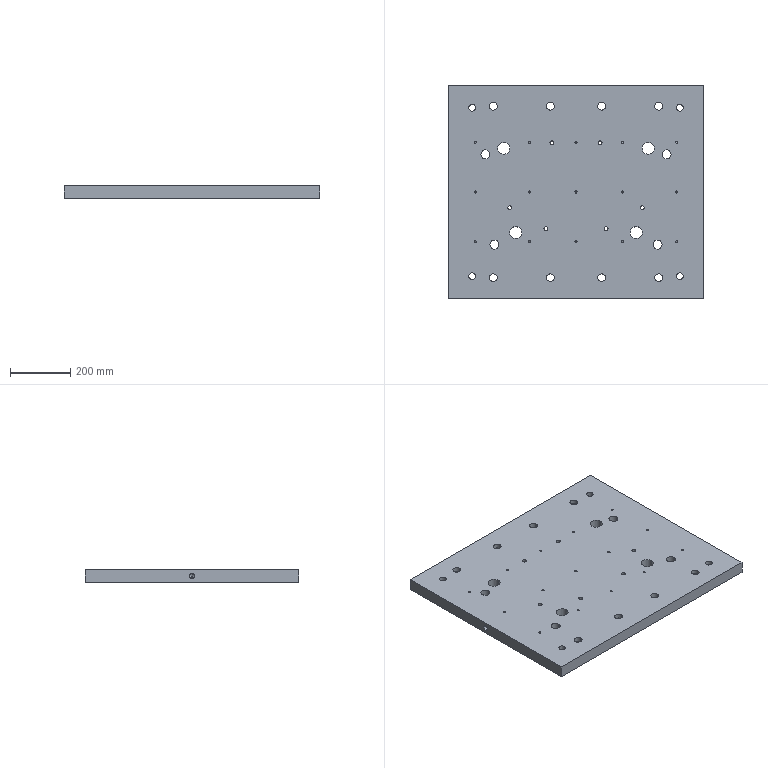Part | SolidWorks | features BaseBody 1 | 1 solid | 206 faces | box 850 x 710 x 40 mm | volume 23346723 mm3 | cylinder 130 | plane 42 | cone 34 | commonest cylinder face diameters 6.8 x30 26 x16 39 x16 13 x12 20 x12 22 x8